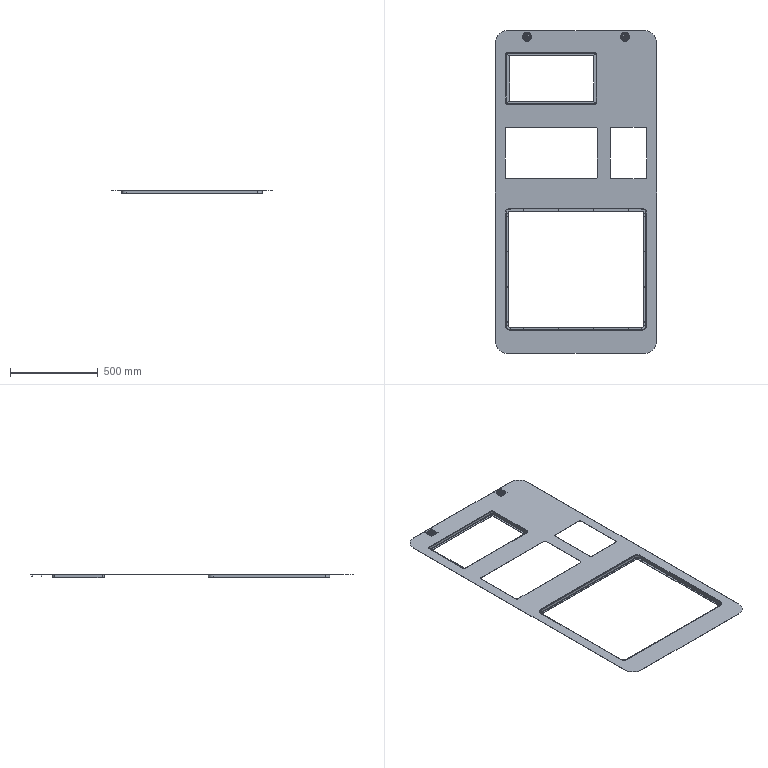Part | STEP file | Split housing part 0201001 | 5 solids | 532 faces | box 920 x 1840 x 21.5 mm | volume 1371751 mm3 | cylinder 280 | plane 220 | torus 32 | commonest cylinder face diameters 4.5 x164 3 x36 3.5 x32 6 x16 20 x12 23 x8